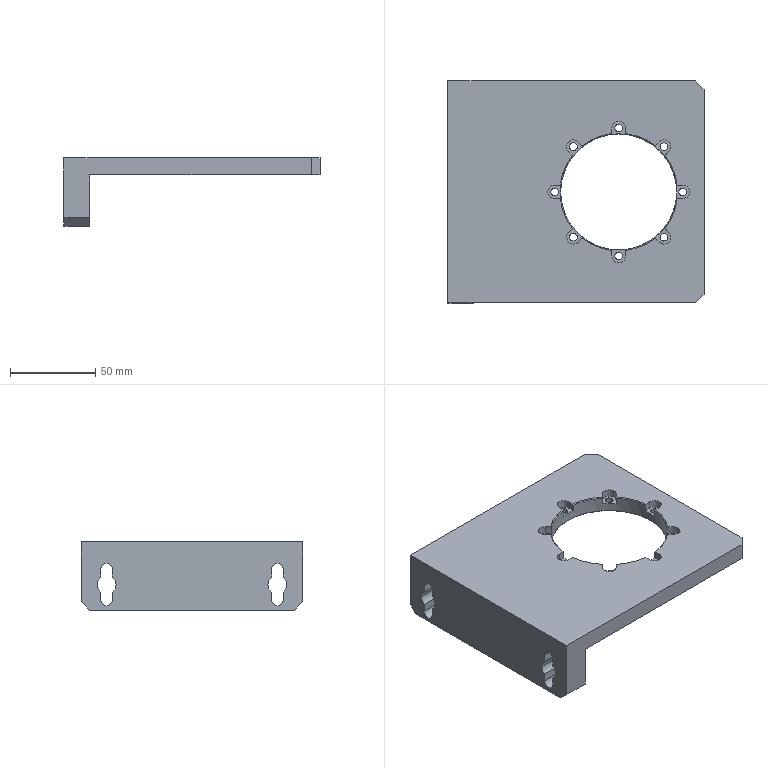NC program | NX | posted with a generic post | part box 150 x 130 x 40 mm
Lines 1 to 823 of 5832:
N10 G17 G21 G94 G90
(ZLEVEL_PROFILE_1 , TOOL : D4)
N12 T11 M6
N14 G54
N16 G17 G0 G90 X-48.599 Y-21.302 B0. C0. S9500 M3
N18 G43 Z30. H11
N20 Z1.5
N22 G94 G1 X-48.614 Y-21.277 Z1.498 F1000.
N24 X-48.724 Y-20.447 Z1.455
N26 X-48.639 Y-20.11 Z1.436
N28 X-48.7 Y-19.975 Z1.429
N30 Y-15.519 Z1.195
N32 X-49.004 Y-14.918 Z1.16
N34 X-49.564 Y-14.544 Z1.125
N36 X-50.235 Y-14.491 Z1.089
N38 X-50.755 Y-14.705 Z1.06
N40 X-51.105 Y-15.06 Z1.034
N42 X-51.3 Y-15.519 Z1.007
N44 Y-20.109 Z0.767
N46 X-51.361 Y-20.11 Z0.764
N48 X-51.276 Y-20.447 Z0.746
N50 X-51.386 Y-21.277 Z0.702
N52 X-51.822 Y-21.991 Z0.658
N54 X-52.467 Y-22.476 Z0.616
N56 X-53.154 Y-23.415 Z0.555
N58 X-53.498 Y-24.526 Z0.494
N60 X-53.502 Y-25.444 Z0.445
N62 X-53.161 Y-26.572 Z0.384
N64 X-52.467 Y-27.524 Z0.322
N66 X-51.822 Y-28.009 Z0.28
N68 X-51.484 Y-28.492 Z0.249
N70 X-51.3 Y-29.052 Z0.218
N72 Y-34.481 Z-0.067
N74 X-51.105 Y-34.94 Z-0.093
N76 X-50.755 Y-35.295 Z-0.119
N78 X-50.235 Y-35.509 Z-0.148
N80 X-49.564 Y-35.456 Z-0.184
N82 X-49.004 Y-35.082 Z-0.219
N84 X-48.7 Y-34.481 Z-0.254
N86 Y-31.8 Z-0.395
N88 Y-29.4 F1400.
N90 G2 X-47.9 Y-27.8 R2.
N92 G3 X-47.9 Y-22.2 R3.5
N94 G2 X-48.639 Y-20.11 R2.
N96 G1 X-48.7 Y-19.975
N98 Y-15.8
N100 G3 X-50. Y-14.5 R1.3
N102 X-51.3 Y-15.8 R1.3
N104 G1 Y-20.048
N106 X-51.296 Y-20.112
N108 X-51.361 Y-20.11
N110 G2 X-52.1 Y-22.2 R2.
N112 G3 X-52.1 Y-27.8 R3.5
N114 G2 X-51.3 Y-29.4 R2.
N116 G1 Y-34.2
N118 G3 X-50. Y-35.5 R1.3
N120 X-48.7 Y-34.2 R1.3
N122 G1 Y-31.8
N124 Y-29.612 Z-0.433
N126 Y-29.368 Z-0.437
N128 X-48.681 Y-29.126 Z-0.441
N130 X-48.633 Y-28.888 Z-0.446
N132 X-48.557 Y-28.657 Z-0.45
N134 X-48.453 Y-28.437 Z-0.454
N136 X-48.323 Y-28.232 Z-0.458
N138 X-48.17 Y-28.044 Z-0.463
N140 X-47.994 Y-27.875 Z-0.467
N142 X-47.803 Y-27.725 Z-0.471
N144 X-47.62 Y-27.566 Z-0.475
N146 X-47.447 Y-27.394 Z-0.48
N148 X-47.287 Y-27.211 Z-0.484
N150 X-47.14 Y-27.018 Z-0.488
N152 X-47.007 Y-26.814 Z-0.492
N154 X-46.888 Y-26.602 Z-0.497
N156 X-46.785 Y-26.382 Z-0.501
N158 X-46.696 Y-26.156 Z-0.505
N160 X-46.624 Y-25.924 Z-0.509
N162 X-46.568 Y-25.687 Z-0.514
N164 X-46.529 Y-25.447 Z-0.518
N166 X-46.506 Y-25.205 Z-0.522
N168 X-46.5 Y-24.962 Z-0.526
N170 X-46.511 Y-24.719 Z-0.531
N172 X-46.539 Y-24.478 Z-0.535
N174 X-46.584 Y-24.239 Z-0.539
N176 X-46.645 Y-24.003 Z-0.543
N178 X-46.722 Y-23.773 Z-0.548
N180 X-46.815 Y-23.548 Z-0.552
N182 X-46.924 Y-23.331 Z-0.556
N184 X-47.047 Y-23.121 Z-0.56
N186 X-47.185 Y-22.921 Z-0.565
N188 X-47.336 Y-22.73 Z-0.569
N190 X-47.5 Y-22.551 Z-0.573
N192 X-47.676 Y-22.383 Z-0.577
N194 X-47.863 Y-22.228 Z-0.581
N196 X-48.051 Y-22.074 Z-0.586
N198 X-48.22 Y-21.9 Z-0.59
N200 X-48.367 Y-21.706 Z-0.594
N202 X-48.488 Y-21.495 Z-0.598
N204 X-48.584 Y-21.272 Z-0.603
N206 X-48.651 Y-21.038 Z-0.607
N208 X-48.69 Y-20.798 Z-0.611
N210 X-48.7 Y-20.556 Z-0.615
N212 X-48.679 Y-20.313 Z-0.62
N214 X-48.654 Y-20.077 Z-0.624
N216 X-48.7 Y-19.844 Z-0.628
N218 Y-15.954 Z-0.696
N220 X-48.703 Y-15.71 Z-0.7
N222 X-48.742 Y-15.471 Z-0.705
N224 X-48.826 Y-15.243 Z-0.709
N226 X-48.95 Y-15.034 Z-0.713
N228 X-49.11 Y-14.852 Z-0.717
N230 X-49.302 Y-14.703 Z-0.722
N232 X-49.518 Y-14.593 Z-0.726
N234 X-49.751 Y-14.524 Z-0.73
N236 X-49.993 Y-14.5 Z-0.734
N238 X-50.235 Y-14.521 Z-0.739
N240 X-50.468 Y-14.587 Z-0.743
N242 X-50.686 Y-14.696 Z-0.747
N244 X-50.879 Y-14.842 Z-0.751
N246 X-51.042 Y-15.023 Z-0.756
N248 X-51.168 Y-15.23 Z-0.76
N250 X-51.254 Y-15.457 Z-0.764
N252 X-51.296 Y-15.696 Z-0.768
N254 X-51.3 Y-15.939 Z-0.772
N256 Y-16.912 Z-0.789
N258 Y-20.048
N260 X-51.296 Y-20.113
N262 X-51.361 Y-20.11
N264 G2 X-52.1 Y-22.2 R2.
N266 G3 X-52.1 Y-27.8 R3.5
N268 G2 X-51.3 Y-29.4 R2.
N270 G1 Y-34.2
N272 G3 X-50. Y-35.5 R1.3
N274 X-48.7 Y-34.2 R1.3
N276 G1 Y-31.8
N278 Y-29.612 Z-0.828
N280 Y-29.368 Z-0.832
N282 X-48.681 Y-29.126 Z-0.836
N284 X-48.633 Y-28.888 Z-0.84
N286 X-48.557 Y-28.657 Z-0.845
N288 X-48.453 Y-28.437 Z-0.849
N290 X-48.323 Y-28.232 Z-0.853
N292 X-48.17 Y-28.044 Z-0.857
N294 X-47.994 Y-27.875 Z-0.862
N296 X-47.803 Y-27.725 Z-0.866
N298 X-47.62 Y-27.566 Z-0.87
N300 X-47.447 Y-27.394 Z-0.874
N302 X-47.287 Y-27.211 Z-0.879
N304 X-47.14 Y-27.018 Z-0.883
N306 X-47.007 Y-26.814 Z-0.887
N308 X-46.888 Y-26.602 Z-0.891
N310 X-46.785 Y-26.382 Z-0.896
N312 X-46.696 Y-26.156 Z-0.9
N314 X-46.624 Y-25.924 Z-0.904
N316 X-46.568 Y-25.687 Z-0.908
N318 X-46.529 Y-25.447 Z-0.913
N320 X-46.506 Y-25.205 Z-0.917
N322 X-46.5 Y-24.962 Z-0.921
N324 X-46.511 Y-24.719 Z-0.925
N326 X-46.539 Y-24.478 Z-0.93
N328 X-46.584 Y-24.239 Z-0.934
N330 X-46.645 Y-24.003 Z-0.938
N332 X-46.722 Y-23.773 Z-0.942
N334 X-46.815 Y-23.548 Z-0.947
N336 X-46.924 Y-23.331 Z-0.951
N338 X-47.047 Y-23.121 Z-0.955
N340 X-47.185 Y-22.921 Z-0.959
N342 X-47.336 Y-22.73 Z-0.963
N344 X-47.5 Y-22.551 Z-0.968
N346 X-47.676 Y-22.383 Z-0.972
N348 X-47.863 Y-22.228 Z-0.976
N350 X-48.051 Y-22.074 Z-0.98
N352 X-48.22 Y-21.9 Z-0.985
N354 X-48.367 Y-21.706 Z-0.989
N356 X-48.488 Y-21.495 Z-0.993
N358 X-48.584 Y-21.272 Z-0.997
N360 X-48.651 Y-21.038 Z-1.002
N362 X-48.69 Y-20.798 Z-1.006
N364 X-48.7 Y-20.556 Z-1.01
N366 X-48.679 Y-20.313 Z-1.014
N368 X-48.654 Y-20.077 Z-1.019
N370 X-48.7 Y-19.844 Z-1.023
N372 Y-15.954 Z-1.091
N374 X-48.703 Y-15.71 Z-1.095
N376 X-48.742 Y-15.471 Z-1.099
N378 X-48.826 Y-15.243 Z-1.104
N380 X-48.95 Y-15.034 Z-1.108
N382 X-49.11 Y-14.852 Z-1.112
N384 X-49.302 Y-14.703 Z-1.116
N386 X-49.518 Y-14.593 Z-1.121
N388 X-49.751 Y-14.524 Z-1.125
N390 X-49.993 Y-14.5 Z-1.129
N392 X-50.235 Y-14.521 Z-1.133
N394 X-50.468 Y-14.587 Z-1.138
N396 X-50.686 Y-14.696 Z-1.142
N398 X-50.879 Y-14.842 Z-1.146
N400 X-51.042 Y-15.023 Z-1.15
N402 X-51.168 Y-15.23 Z-1.155
N404 X-51.254 Y-15.457 Z-1.159
N406 X-51.296 Y-15.696 Z-1.163
N408 X-51.3 Y-15.939 Z-1.167
N410 Y-16.912 Z-1.184
N412 Y-20.048
N414 X-51.296 Y-20.113
N416 X-51.361 Y-20.11
N418 G2 X-52.1 Y-22.2 R2.
N420 G3 X-52.1 Y-27.8 R3.5
N422 G2 X-51.3 Y-29.4 R2.
N424 G1 Y-34.2
N426 G3 X-50. Y-35.5 R1.3
N428 X-48.7 Y-34.2 R1.3
N430 G1 Y-31.8
N432 Y-29.612 Z-1.222
N434 Y-29.368 Z-1.227
N436 X-48.681 Y-29.126 Z-1.231
N438 X-48.633 Y-28.888 Z-1.235
N440 X-48.557 Y-28.657 Z-1.239
N442 X-48.453 Y-28.437 Z-1.244
N444 X-48.323 Y-28.232 Z-1.248
N446 X-48.17 Y-28.044 Z-1.252
N448 X-47.994 Y-27.875 Z-1.256
N450 X-47.803 Y-27.725 Z-1.261
N452 X-47.62 Y-27.566 Z-1.265
N454 X-47.447 Y-27.394 Z-1.269
N456 X-47.287 Y-27.211 Z-1.273
N458 X-47.14 Y-27.018 Z-1.278
N460 X-47.007 Y-26.814 Z-1.282
N462 X-46.888 Y-26.602 Z-1.286
N464 X-46.785 Y-26.382 Z-1.29
N466 X-46.696 Y-26.156 Z-1.295
N468 X-46.624 Y-25.924 Z-1.299
N470 X-46.568 Y-25.687 Z-1.303
N472 X-46.529 Y-25.447 Z-1.307
N474 X-46.506 Y-25.205 Z-1.312
N476 X-46.5 Y-24.962 Z-1.316
N478 X-46.511 Y-24.719 Z-1.32
N480 X-46.539 Y-24.478 Z-1.324
N482 X-46.584 Y-24.239 Z-1.329
N484 X-46.645 Y-24.003 Z-1.333
N486 X-46.722 Y-23.773 Z-1.337
N488 X-46.815 Y-23.548 Z-1.341
N490 X-46.924 Y-23.331 Z-1.346
N492 X-47.047 Y-23.121 Z-1.35
N494 X-47.185 Y-22.921 Z-1.354
N496 X-47.336 Y-22.73 Z-1.358
N498 X-47.5 Y-22.551 Z-1.362
N500 X-47.676 Y-22.383 Z-1.367
N502 X-47.863 Y-22.228 Z-1.371
N504 X-48.051 Y-22.074 Z-1.375
N506 X-48.22 Y-21.9 Z-1.379
N508 X-48.367 Y-21.706 Z-1.384
N510 X-48.488 Y-21.495 Z-1.388
N512 X-48.584 Y-21.272 Z-1.392
N514 X-48.651 Y-21.038 Z-1.396
N516 X-48.69 Y-20.798 Z-1.401
N518 X-48.7 Y-20.556 Z-1.405
N520 X-48.679 Y-20.313 Z-1.409
N522 X-48.654 Y-20.077 Z-1.413
N524 X-48.7 Y-19.844 Z-1.418
N526 Y-15.954 Z-1.486
N528 X-48.703 Y-15.71 Z-1.49
N530 X-48.742 Y-15.471 Z-1.494
N532 X-48.826 Y-15.243 Z-1.498
N534 X-48.95 Y-15.034 Z-1.503
N536 X-49.11 Y-14.852 Z-1.507
N538 X-49.302 Y-14.703 Z-1.511
N540 X-49.518 Y-14.593 Z-1.515
N542 X-49.751 Y-14.524 Z-1.52
N544 X-49.993 Y-14.5 Z-1.524
N546 X-50.235 Y-14.521 Z-1.528
N548 X-50.468 Y-14.587 Z-1.532
N550 X-50.686 Y-14.696 Z-1.537
N552 X-50.879 Y-14.842 Z-1.541
N554 X-51.042 Y-15.023 Z-1.545
N556 X-51.168 Y-15.23 Z-1.549
N558 X-51.254 Y-15.457 Z-1.553
N560 X-51.296 Y-15.696 Z-1.558
N562 X-51.3 Y-15.939 Z-1.562
N564 Y-16.912 Z-1.579
N566 Y-20.049
N568 X-51.297 Y-20.113
N570 X-51.361 Y-20.11
N572 G2 X-52.1 Y-22.2 R2.
N574 G3 X-52.1 Y-27.8 R3.5
N576 G2 X-51.3 Y-29.4 R2.
N578 G1 Y-34.2
N580 G3 X-50. Y-35.5 R1.3
N582 X-48.7 Y-34.2 R1.3
N584 G1 Y-31.8
N586 Y-29.612 Z-1.617
N588 Y-29.368 Z-1.621
N590 X-48.681 Y-29.126 Z-1.626
N592 X-48.633 Y-28.888 Z-1.63
N594 X-48.557 Y-28.657 Z-1.634
N596 X-48.453 Y-28.437 Z-1.638
N598 X-48.323 Y-28.232 Z-1.643
N600 X-48.17 Y-28.044 Z-1.647
N602 X-47.994 Y-27.875 Z-1.651
N604 X-47.803 Y-27.725 Z-1.655
N606 X-47.62 Y-27.566 Z-1.66
N608 X-47.447 Y-27.394 Z-1.664
N610 X-47.287 Y-27.211 Z-1.668
N612 X-47.14 Y-27.018 Z-1.672
N614 X-47.007 Y-26.814 Z-1.677
N616 X-46.888 Y-26.602 Z-1.681
N618 X-46.785 Y-26.382 Z-1.685
N620 X-46.696 Y-26.156 Z-1.689
N622 X-46.624 Y-25.924 Z-1.694
N624 X-46.568 Y-25.687 Z-1.698
N626 X-46.529 Y-25.447 Z-1.702
N628 X-46.506 Y-25.205 Z-1.706
N630 X-46.5 Y-24.962 Z-1.711
N632 X-46.511 Y-24.719 Z-1.715
N634 X-46.539 Y-24.478 Z-1.719
N636 X-46.584 Y-24.239 Z-1.723
N638 X-46.645 Y-24.003 Z-1.728
N640 X-46.722 Y-23.773 Z-1.732
N642 X-46.815 Y-23.548 Z-1.736
N644 X-46.924 Y-23.331 Z-1.74
N646 X-47.047 Y-23.121 Z-1.744
N648 X-47.185 Y-22.921 Z-1.749
N650 X-47.336 Y-22.73 Z-1.753
N652 X-47.5 Y-22.551 Z-1.757
N654 X-47.676 Y-22.383 Z-1.761
N656 X-47.863 Y-22.228 Z-1.766
N658 X-48.051 Y-22.074 Z-1.77
N660 X-48.22 Y-21.9 Z-1.774
N662 X-48.367 Y-21.706 Z-1.778
N664 X-48.488 Y-21.495 Z-1.783
N666 X-48.584 Y-21.272 Z-1.787
N668 X-48.651 Y-21.038 Z-1.791
N670 X-48.69 Y-20.798 Z-1.795
N672 X-48.7 Y-20.556 Z-1.8
N674 X-48.679 Y-20.313 Z-1.804
N676 X-48.654 Y-20.077 Z-1.808
N678 X-48.7 Y-19.844 Z-1.812
N680 Y-15.954 Z-1.88
N682 X-48.703 Y-15.71 Z-1.885
N684 X-48.742 Y-15.471 Z-1.889
N686 X-48.826 Y-15.243 Z-1.893
N688 X-48.95 Y-15.034 Z-1.897
N690 X-49.11 Y-14.852 Z-1.902
N692 X-49.302 Y-14.703 Z-1.906
N694 X-49.518 Y-14.593 Z-1.91
N696 X-49.751 Y-14.524 Z-1.914
N698 X-49.993 Y-14.5 Z-1.919
N700 X-50.235 Y-14.521 Z-1.923
N702 X-50.468 Y-14.587 Z-1.927
N704 X-50.686 Y-14.696 Z-1.931
N706 X-50.879 Y-14.842 Z-1.935
N708 X-51.042 Y-15.023 Z-1.94
N710 X-51.168 Y-15.23 Z-1.944
N712 X-51.254 Y-15.457 Z-1.948
N714 X-51.296 Y-15.696 Z-1.952
N716 X-51.3 Y-15.939 Z-1.957
N718 Y-16.912 Z-1.974
N720 Y-20.049
N722 X-51.297 Y-20.113
N724 X-51.361 Y-20.11
N726 G2 X-52.1 Y-22.2 R2.
N728 G3 X-52.1 Y-27.8 R3.5
N730 G2 X-51.3 Y-29.4 R2.
N732 G1 Y-34.2
N734 G3 X-50. Y-35.5 R1.3
N736 X-48.7 Y-34.2 R1.3
N738 G1 Y-31.8
N740 Y-29.612 Z-2.012
N742 Y-29.368 Z-2.016
N744 X-48.681 Y-29.126 Z-2.02
N746 X-48.633 Y-28.888 Z-2.025
N748 X-48.557 Y-28.657 Z-2.029
N750 X-48.453 Y-28.437 Z-2.033
N752 X-48.323 Y-28.232 Z-2.037
N754 X-48.17 Y-28.044 Z-2.042
N756 X-47.994 Y-27.875 Z-2.046
N758 X-47.803 Y-27.725 Z-2.05
N760 X-47.62 Y-27.566 Z-2.054
N762 X-47.447 Y-27.394 Z-2.059
N764 X-47.287 Y-27.211 Z-2.063
N766 X-47.14 Y-27.018 Z-2.067
N768 X-47.007 Y-26.814 Z-2.071
N770 X-46.888 Y-26.602 Z-2.076
N772 X-46.785 Y-26.382 Z-2.08
N774 X-46.696 Y-26.156 Z-2.084
N776 X-46.624 Y-25.924 Z-2.088
N778 X-46.568 Y-25.687 Z-2.093
N780 X-46.529 Y-25.447 Z-2.097
N782 X-46.506 Y-25.205 Z-2.101
N784 X-46.5 Y-24.962 Z-2.105
N786 X-46.511 Y-24.719 Z-2.11
N788 X-46.539 Y-24.478 Z-2.114
N790 X-46.584 Y-24.239 Z-2.118
N792 X-46.645 Y-24.003 Z-2.122
N794 X-46.722 Y-23.773 Z-2.126
N796 X-46.815 Y-23.548 Z-2.131
N798 X-46.924 Y-23.331 Z-2.135
N800 X-47.047 Y-23.121 Z-2.139
N802 X-47.185 Y-22.921 Z-2.143
N804 X-47.336 Y-22.73 Z-2.148
N806 X-47.5 Y-22.551 Z-2.152
N808 X-47.676 Y-22.383 Z-2.156
N810 X-47.863 Y-22.228 Z-2.16
N812 X-48.051 Y-22.074 Z-2.165
N814 X-48.22 Y-21.9 Z-2.169
N816 X-48.367 Y-21.706 Z-2.173
N818 X-48.488 Y-21.495 Z-2.177
N820 X-48.584 Y-21.272 Z-2.182
N822 X-48.651 Y-21.038 Z-2.186
N824 X-48.69 Y-20.798 Z-2.19
N826 X-48.7 Y-20.556 Z-2.194
N828 X-48.679 Y-20.313 Z-2.199
N830 X-48.654 Y-20.077 Z-2.203
N832 X-48.7 Y-19.844 Z-2.207
N834 Y-15.954 Z-2.275
N836 X-48.703 Y-15.71 Z-2.279
N838 X-48.742 Y-15.471 Z-2.284
N840 X-48.826 Y-15.243 Z-2.288
N842 X-48.95 Y-15.034 Z-2.292
N844 X-49.11 Y-14.852 Z-2.296
N846 X-49.302 Y-14.703 Z-2.301
N848 X-49.518 Y-14.593 Z-2.305
N850 X-49.751 Y-14.524 Z-2.309
N852 X-49.993 Y-14.5 Z-2.313
N854 X-50.235 Y-14.521 Z-2.317
N856 X-50.468 Y-14.587 Z-2.322
N858 X-50.686 Y-14.696 Z-2.326
N860 X-50.879 Y-14.842 Z-2.33
N862 X-51.042 Y-15.023 Z-2.334
N864 X-51.168 Y-15.23 Z-2.339
N866 X-51.254 Y-15.457 Z-2.343
N868 X-51.296 Y-15.696 Z-2.347
N870 X-51.3 Y-15.939 Z-2.351
N872 Y-16.912 Z-2.368
N874 Y-20.049
N876 X-51.297 Y-20.114
N878 X-51.361 Y-20.11
N880 G2 X-52.1 Y-22.2 R2.
N882 G3 X-52.1 Y-27.8 R3.5
N884 G2 X-51.3 Y-29.4 R2.
N886 G1 Y-34.2
N888 G3 X-50. Y-35.5 R1.3
N890 X-48.7 Y-34.2 R1.3
N892 G1 Y-31.8
N894 Y-29.612 Z-2.407
N896 Y-29.368 Z-2.411
N898 X-48.681 Y-29.126 Z-2.415
N900 X-48.633 Y-28.888 Z-2.419
N902 X-48.557 Y-28.657 Z-2.424
N904 X-48.453 Y-28.437 Z-2.428
N906 X-48.323 Y-28.232 Z-2.432
N908 X-48.17 Y-28.044 Z-2.436
N910 X-47.994 Y-27.875 Z-2.441
N912 X-47.803 Y-27.725 Z-2.445
N914 X-47.62 Y-27.566 Z-2.449
N916 X-47.447 Y-27.394 Z-2.453
N918 X-47.287 Y-27.211 Z-2.458
N920 X-47.14 Y-27.018 Z-2.462
N922 X-47.007 Y-26.814 Z-2.466
N924 X-46.888 Y-26.602 Z-2.47
N926 X-46.785 Y-26.382 Z-2.475
N928 X-46.696 Y-26.156 Z-2.479
N930 X-46.624 Y-25.924 Z-2.483
N932 X-46.568 Y-25.687 Z-2.487
N934 X-46.529 Y-25.447 Z-2.492
N936 X-46.506 Y-25.205 Z-2.496
N938 X-46.5 Y-24.962 Z-2.5
N940 X-46.511 Y-24.719 Z-2.504
N942 X-46.539 Y-24.478 Z-2.508
N944 X-46.584 Y-24.239 Z-2.513
N946 X-46.645 Y-24.003 Z-2.517
N948 X-46.722 Y-23.773 Z-2.521
N950 X-46.815 Y-23.548 Z-2.525
N952 X-46.924 Y-23.331 Z-2.53
N954 X-47.047 Y-23.121 Z-2.534
N956 X-47.185 Y-22.921 Z-2.538
N958 X-47.336 Y-22.73 Z-2.542
N960 X-47.5 Y-22.551 Z-2.547
N962 X-47.676 Y-22.383 Z-2.551
N964 X-47.863 Y-22.228 Z-2.555
N966 X-48.051 Y-22.074 Z-2.559
N968 X-48.22 Y-21.9 Z-2.564
N970 X-48.367 Y-21.706 Z-2.568
N972 X-48.488 Y-21.495 Z-2.572
N974 X-48.584 Y-21.272 Z-2.576
N976 X-48.651 Y-21.038 Z-2.581
N978 X-48.69 Y-20.798 Z-2.585
N980 X-48.7 Y-20.556 Z-2.589
N982 X-48.679 Y-20.313 Z-2.593
N984 X-48.654 Y-20.077 Z-2.598
N986 X-48.7 Y-19.844 Z-2.602
N988 Y-15.954 Z-2.67
N990 X-48.703 Y-15.71 Z-2.674
N992 X-48.742 Y-15.471 Z-2.678
N994 X-48.826 Y-15.243 Z-2.683
N996 X-48.95 Y-15.034 Z-2.687
N998 X-49.11 Y-14.852 Z-2.691
N1000 X-49.302 Y-14.703 Z-2.695
N1002 X-49.518 Y-14.593 Z-2.699
N1004 X-49.751 Y-14.524 Z-2.704
N1006 X-49.993 Y-14.5 Z-2.708
N1008 X-50.235 Y-14.521 Z-2.712
N1010 X-50.468 Y-14.587 Z-2.716
N1012 X-50.686 Y-14.696 Z-2.721
N1014 X-50.879 Y-14.842 Z-2.725
N1016 X-51.042 Y-15.023 Z-2.729
N1018 X-51.168 Y-15.23 Z-2.733
N1020 X-51.254 Y-15.457 Z-2.738
N1022 X-51.296 Y-15.696 Z-2.742
N1024 X-51.3 Y-15.939 Z-2.746
N1026 Y-16.912 Z-2.763
N1028 Y-20.05
N1030 X-51.297 Y-20.114
N1032 X-51.361 Y-20.11
N1034 G2 X-52.1 Y-22.2 R2.
N1036 G3 X-52.1 Y-27.8 R3.5
N1038 G2 X-51.3 Y-29.4 R2.
N1040 G1 Y-34.2
N1042 G3 X-50. Y-35.5 R1.3
N1044 X-48.7 Y-34.2 R1.3
N1046 G1 Y-31.8
N1048 Y-29.612 Z-2.801
N1050 Y-29.368 Z-2.806
N1052 X-48.681 Y-29.126 Z-2.81
N1054 X-48.633 Y-28.888 Z-2.814
N1056 X-48.557 Y-28.657 Z-2.818
N1058 X-48.453 Y-28.437 Z-2.823
N1060 X-48.323 Y-28.232 Z-2.827
N1062 X-48.17 Y-28.044 Z-2.831
N1064 X-47.994 Y-27.875 Z-2.835
N1066 X-47.803 Y-27.725 Z-2.84
N1068 X-47.62 Y-27.566 Z-2.844
N1070 X-47.447 Y-27.394 Z-2.848
N1072 X-47.287 Y-27.211 Z-2.852
N1074 X-47.14 Y-27.018 Z-2.857
N1076 X-47.007 Y-26.814 Z-2.861
N1078 X-46.888 Y-26.602 Z-2.865
N1080 X-46.785 Y-26.382 Z-2.869
N1082 X-46.696 Y-26.156 Z-2.874
N1084 X-46.624 Y-25.924 Z-2.878
N1086 X-46.568 Y-25.687 Z-2.882
N1088 X-46.529 Y-25.447 Z-2.886
N1090 X-46.506 Y-25.205 Z-2.89
N1092 X-46.5 Y-24.962 Z-2.895
N1094 X-46.511 Y-24.719 Z-2.899
N1096 X-46.539 Y-24.478 Z-2.903
N1098 X-46.584 Y-24.239 Z-2.907
N1100 X-46.645 Y-24.003 Z-2.912
N1102 X-46.722 Y-23.773 Z-2.916
N1104 X-46.815 Y-23.548 Z-2.92
N1106 X-46.924 Y-23.331 Z-2.924
N1108 X-47.047 Y-23.121 Z-2.929
N1110 X-47.185 Y-22.921 Z-2.933
N1112 X-47.336 Y-22.73 Z-2.937
N1114 X-47.5 Y-22.551 Z-2.941
N1116 X-47.676 Y-22.383 Z-2.946
N1118 X-47.863 Y-22.228 Z-2.95
N1120 X-48.051 Y-22.074 Z-2.954
N1122 X-48.22 Y-21.9 Z-2.958
N1124 X-48.367 Y-21.706 Z-2.963
N1126 X-48.488 Y-21.495 Z-2.967
N1128 X-48.584 Y-21.272 Z-2.971
N1130 X-48.651 Y-21.038 Z-2.975
N1132 X-48.69 Y-20.798 Z-2.98
N1134 X-48.7 Y-20.556 Z-2.984
N1136 X-48.679 Y-20.313 Z-2.988
N1138 X-48.654 Y-20.077 Z-2.992
N1140 X-48.7 Y-19.844 Z-2.997
N1142 Y-15.954 Z-3.065
N1144 X-48.703 Y-15.71 Z-3.069
N1146 X-48.742 Y-15.471 Z-3.073
N1148 X-48.826 Y-15.243 Z-3.077
N1150 X-48.95 Y-15.034 Z-3.081
N1152 X-49.11 Y-14.852 Z-3.086
N1154 X-49.302 Y-14.703 Z-3.09
N1156 X-49.518 Y-14.593 Z-3.094
N1158 X-49.751 Y-14.524 Z-3.098
N1160 X-49.993 Y-14.5 Z-3.103
N1162 X-50.235 Y-14.521 Z-3.107
N1164 X-50.468 Y-14.587 Z-3.111
N1166 X-50.686 Y-14.696 Z-3.115
N1168 X-50.879 Y-14.842 Z-3.12
N1170 X-51.042 Y-15.023 Z-3.124
N1172 X-51.168 Y-15.23 Z-3.128
N1174 X-51.254 Y-15.457 Z-3.132
N1176 X-51.296 Y-15.696 Z-3.137
N1178 X-51.3 Y-15.939 Z-3.141
N1180 Y-16.912 Z-3.158
N1182 Y-20.05
N1184 X-51.297 Y-20.114
N1186 X-51.361 Y-20.11
N1188 G2 X-52.1 Y-22.2 R2.
N1190 G3 X-52.1 Y-27.8 R3.5
N1192 G2 X-51.3 Y-29.4 R2.
N1194 G1 Y-34.2
N1196 G3 X-50. Y-35.5 R1.3
N1198 X-48.7 Y-34.2 R1.3
N1200 G1 Y-31.8
N1202 Y-29.612 Z-3.196
N1204 Y-29.368 Z-3.2
N1206 X-48.681 Y-29.126 Z-3.205
N1208 X-48.633 Y-28.888 Z-3.209
N1210 X-48.557 Y-28.657 Z-3.213
N1212 X-48.453 Y-28.437 Z-3.217
N1214 X-48.323 Y-28.232 Z-3.222
N1216 X-48.17 Y-28.044 Z-3.226
N1218 X-47.994 Y-27.875 Z-3.23
N1220 X-47.803 Y-27.725 Z-3.234
N1222 X-47.62 Y-27.566 Z-3.239
N1224 X-47.447 Y-27.394 Z-3.243
N1226 X-47.287 Y-27.211 Z-3.247
N1228 X-47.14 Y-27.018 Z-3.251
N1230 X-47.007 Y-26.814 Z-3.256
N1232 X-46.888 Y-26.602 Z-3.26
N1234 X-46.785 Y-26.382 Z-3.264
N1236 X-46.696 Y-26.156 Z-3.268
N1238 X-46.624 Y-25.924 Z-3.272
N1240 X-46.568 Y-25.687 Z-3.277
N1242 X-46.529 Y-25.447 Z-3.281
N1244 X-46.506 Y-25.205 Z-3.285
N1246 X-46.5 Y-24.962 Z-3.289
N1248 X-46.511 Y-24.719 Z-3.294
N1250 X-46.539 Y-24.478 Z-3.298
N1252 X-46.584 Y-24.239 Z-3.302
N1254 X-46.645 Y-24.003 Z-3.306
N1256 X-46.722 Y-23.773 Z-3.311
N1258 X-46.815 Y-23.548 Z-3.315
N1260 X-46.924 Y-23.331 Z-3.319
N1262 X-47.047 Y-23.121 Z-3.323
N1264 X-47.185 Y-22.921 Z-3.328
N1266 X-47.336 Y-22.73 Z-3.332
N1268 X-47.5 Y-22.551 Z-3.336
N1270 X-47.676 Y-22.383 Z-3.34
N1272 X-47.863 Y-22.228 Z-3.345
N1274 X-48.051 Y-22.074 Z-3.349
N1276 X-48.22 Y-21.9 Z-3.353
N1278 X-48.367 Y-21.706 Z-3.357
N1280 X-48.488 Y-21.495 Z-3.362
N1282 X-48.584 Y-21.272 Z-3.366
N1284 X-48.651 Y-21.038 Z-3.37
N1286 X-48.69 Y-20.798 Z-3.374
N1288 X-48.7 Y-20.556 Z-3.379
N1290 X-48.679 Y-20.313 Z-3.383
N1292 X-48.654 Y-20.077 Z-3.387
N1294 X-48.7 Y-19.844 Z-3.391
N1296 Y-15.954 Z-3.459
N1298 X-48.703 Y-15.71 Z-3.463
N1300 X-48.742 Y-15.471 Z-3.468
N1302 X-48.826 Y-15.243 Z-3.472
N1304 X-48.95 Y-15.034 Z-3.476
N1306 X-49.11 Y-14.852 Z-3.48
N1308 X-49.302 Y-14.703 Z-3.485
N1310 X-49.518 Y-14.593 Z-3.489
N1312 X-49.751 Y-14.524 Z-3.493
N1314 X-49.993 Y-14.5 Z-3.497
N1316 X-50.235 Y-14.521 Z-3.502
N1318 X-50.468 Y-14.587 Z-3.506
N1320 X-50.686 Y-14.696 Z-3.51
N1322 X-50.879 Y-14.842 Z-3.514
N1324 X-51.042 Y-15.023 Z-3.519
N1326 X-51.168 Y-15.23 Z-3.523
N1328 X-51.254 Y-15.457 Z-3.527
N1330 X-51.296 Y-15.696 Z-3.531
N1332 X-51.3 Y-15.939 Z-3.536
N1334 Y-16.912 Z-3.553
N1336 Y-20.05
N1338 X-51.297 Y-20.114
N1340 X-51.361 Y-20.11
N1342 G2 X-52.1 Y-22.2 R2.
N1344 G3 X-52.1 Y-27.8 R3.5
N1346 G2 X-51.3 Y-29.4 R2.
N1348 G1 Y-34.2
N1350 G3 X-50. Y-35.5 R1.3
N1352 X-48.7 Y-34.2 R1.3
N1354 G1 Y-31.8
N1356 Y-29.612 Z-3.591
N1358 Y-29.368 Z-3.595
N1360 X-48.681 Y-29.126 Z-3.599
N1362 X-48.633 Y-28.888 Z-3.604
N1364 X-48.557 Y-28.657 Z-3.608
N1366 X-48.453 Y-28.437 Z-3.612
N1368 X-48.323 Y-28.232 Z-3.616
N1370 X-48.17 Y-28.044 Z-3.621
N1372 X-47.994 Y-27.875 Z-3.625
N1374 X-47.803 Y-27.725 Z-3.629
N1376 X-47.62 Y-27.566 Z-3.633
N1378 X-47.447 Y-27.394 Z-3.638
N1380 X-47.287 Y-27.211 Z-3.642
N1382 X-47.14 Y-27.018 Z-3.646
N1384 X-47.007 Y-26.814 Z-3.65
N1386 X-46.888 Y-26.602 Z-3.655
N1388 X-46.785 Y-26.382 Z-3.659
N1390 X-46.696 Y-26.156 Z-3.663
N1392 X-46.624 Y-25.924 Z-3.667
N1394 X-46.568 Y-25.687 Z-3.671
N1396 X-46.529 Y-25.447 Z-3.676
N1398 X-46.506 Y-25.205 Z-3.68
N1400 X-46.5 Y-24.962 Z-3.684
N1402 X-46.511 Y-24.719 Z-3.688
N1404 X-46.539 Y-24.478 Z-3.693
N1406 X-46.584 Y-24.239 Z-3.697
N1408 X-46.645 Y-24.003 Z-3.701
N1410 X-46.722 Y-23.773 Z-3.705
N1412 X-46.815 Y-23.548 Z-3.71
N1414 X-46.924 Y-23.331 Z-3.714
N1416 X-47.047 Y-23.121 Z-3.718
N1418 X-47.185 Y-22.921 Z-3.722
N1420 X-47.336 Y-22.73 Z-3.727
N1422 X-47.5 Y-22.551 Z-3.731
N1424 X-47.676 Y-22.383 Z-3.735
N1426 X-47.863 Y-22.228 Z-3.739
N1428 X-48.051 Y-22.074 Z-3.744
N1430 X-48.22 Y-21.9 Z-3.748
N1432 X-48.367 Y-21.706 Z-3.752
N1434 X-48.488 Y-21.495 Z-3.756
N1436 X-48.584 Y-21.272 Z-3.761
N1438 X-48.651 Y-21.038 Z-3.765
N1440 X-48.69 Y-20.798 Z-3.769
N1442 X-48.7 Y-20.556 Z-3.773
N1444 X-48.679 Y-20.313 Z-3.778
N1446 X-48.654 Y-20.077 Z-3.782
N1448 X-48.7 Y-19.844 Z-3.786
N1450 Y-15.954 Z-3.854
N1452 X-48.703 Y-15.71 Z-3.858
N1454 X-48.742 Y-15.471 Z-3.862
N1456 X-48.826 Y-15.243 Z-3.867
N1458 X-48.95 Y-15.034 Z-3.871
N1460 X-49.11 Y-14.852 Z-3.875
N1462 X-49.302 Y-14.703 Z-3.879
N1464 X-49.518 Y-14.593 Z-3.884
N1466 X-49.751 Y-14.524 Z-3.888
N1468 X-49.993 Y-14.5 Z-3.892
N1470 X-50.235 Y-14.521 Z-3.896
N1472 X-50.468 Y-14.587 Z-3.901
N1474 X-50.686 Y-14.696 Z-3.905
N1476 X-50.879 Y-14.842 Z-3.909
N1478 X-51.042 Y-15.023 Z-3.913
N1480 X-51.168 Y-15.23 Z-3.918
N1482 X-51.254 Y-15.457 Z-3.922
N1484 X-51.296 Y-15.696 Z-3.926
N1486 X-51.3 Y-15.939 Z-3.93
N1488 Y-16.912 Z-3.947
N1490 Y-20.051
N1492 X-51.297 Y-20.115
N1494 X-51.361 Y-20.11
N1496 G2 X-52.1 Y-22.2 R2.
N1498 G3 X-52.1 Y-27.8 R3.5
N1500 G2 X-51.3 Y-29.4 R2.
N1502 G1 Y-34.2
N1504 G3 X-50. Y-35.5 R1.3
N1506 X-48.7 Y-34.2 R1.3
N1508 G1 Y-31.8
N1510 Y-29.612 Z-3.986
N1512 Y-29.368 Z-3.99
N1514 X-48.681 Y-29.126 Z-3.994
N1516 X-48.633 Y-28.888 Z-3.998
N1518 X-48.557 Y-28.657 Z-4.003
N1520 X-48.453 Y-28.437 Z-4.007
N1522 X-48.323 Y-28.232 Z-4.011
N1524 X-48.17 Y-28.044 Z-4.015
N1526 X-47.994 Y-27.875 Z-4.02
N1528 X-47.803 Y-27.725 Z-4.024
N1530 X-47.62 Y-27.566 Z-4.028
N1532 X-47.447 Y-27.394 Z-4.032
N1534 X-47.287 Y-27.211 Z-4.037
N1536 X-47.14 Y-27.018 Z-4.041
N1538 X-47.007 Y-26.814 Z-4.045
N1540 X-46.888 Y-26.602 Z-4.049
N1542 X-46.785 Y-26.382 Z-4.053
N1544 X-46.696 Y-26.156 Z-4.058
N1546 X-46.624 Y-25.924 Z-4.062
N1548 X-46.568 Y-25.687 Z-4.066
N1550 X-46.529 Y-25.447 Z-4.07
N1552 X-46.506 Y-25.205 Z-4.075
N1554 X-46.5 Y-24.962 Z-4.079
N1556 X-46.511 Y-24.719 Z-4.083
N1558 X-46.539 Y-24.478 Z-4.087
N1560 X-46.584 Y-24.239 Z-4.092
N1562 X-46.645 Y-24.003 Z-4.096
N1564 X-46.722 Y-23.773 Z-4.1
N1566 X-46.815 Y-23.548 Z-4.104
N1568 X-46.924 Y-23.331 Z-4.109
N1570 X-47.047 Y-23.121 Z-4.113
N1572 X-47.185 Y-22.921 Z-4.117
N1574 X-47.336 Y-22.73 Z-4.121
N1576 X-47.5 Y-22.551 Z-4.126
N1578 X-47.676 Y-22.383 Z-4.13
N1580 X-47.863 Y-22.228 Z-4.134
N1582 X-48.051 Y-22.074 Z-4.138
N1584 X-48.22 Y-21.9 Z-4.143
N1586 X-48.367 Y-21.706 Z-4.147
N1588 X-48.488 Y-21.495 Z-4.151
N1590 X-48.584 Y-21.272 Z-4.155
N1592 X-48.651 Y-21.038 Z-4.16
N1594 X-48.69 Y-20.798 Z-4.164
N1596 X-48.7 Y-20.556 Z-4.168
N1598 X-48.679 Y-20.313 Z-4.172
N1600 X-48.654 Y-20.077 Z-4.177
N1602 X-48.7 Y-19.844 Z-4.181
N1604 Y-15.954 Z-4.249
N1606 X-48.703 Y-15.71 Z-4.253
N1608 X-48.742 Y-15.471 Z-4.257
N1610 X-48.826 Y-15.243 Z-4.261
N1612 X-48.95 Y-15.034 Z-4.266
N1614 X-49.11 Y-14.852 Z-4.27
N1616 X-49.302 Y-14.703 Z-4.274
N1618 X-49.518 Y-14.593 Z-4.278
N1620 X-49.751 Y-14.524 Z-4.283
N1622 X-49.993 Y-14.5 Z-4.287
N1624 X-50.235 Y-14.521 Z-4.291
N1626 X-50.468 Y-14.587 Z-4.295
N1628 X-50.686 Y-14.696 Z-4.3
N1630 X-50.879 Y-14.842 Z-4.304
N1632 X-51.042 Y-15.023 Z-4.308
N1634 X-51.168 Y-15.23 Z-4.312
N1636 X-51.254 Y-15.457 Z-4.317
N1638 X-51.296 Y-15.696 Z-4.321
N1640 X-51.3 Y-15.939 Z-4.325
N1642 Y-16.912 Z-4.342
N1644 Y-20.051